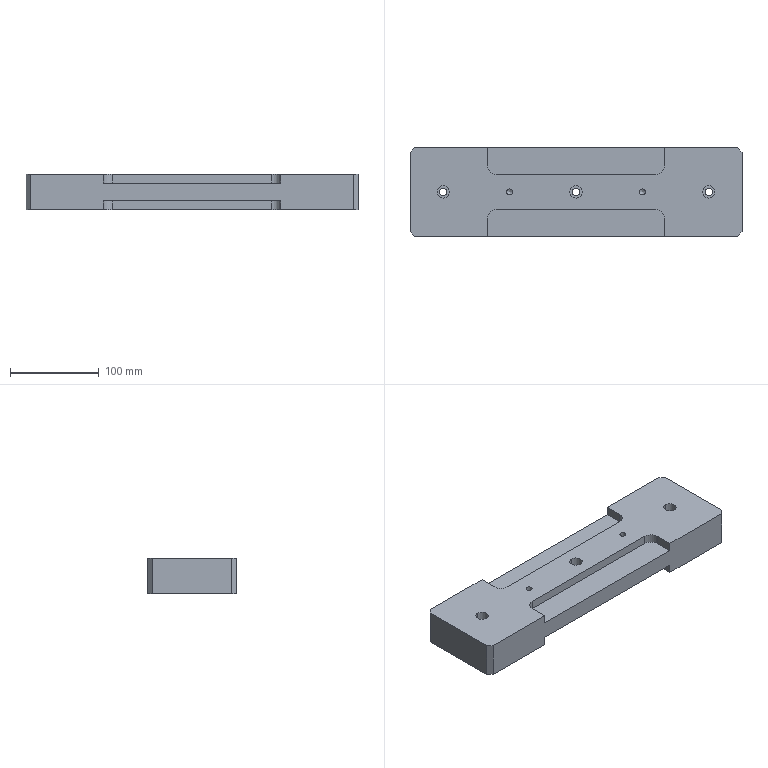Part | 1 solid | 57 faces | box 375 x 100 x 40 mm | volume 1245592 mm3 | plane 29 | cylinder 24 | cone 4 | commonest cylinder face diameters 20 x8 8.5 x6 14 x6 6.8 x4